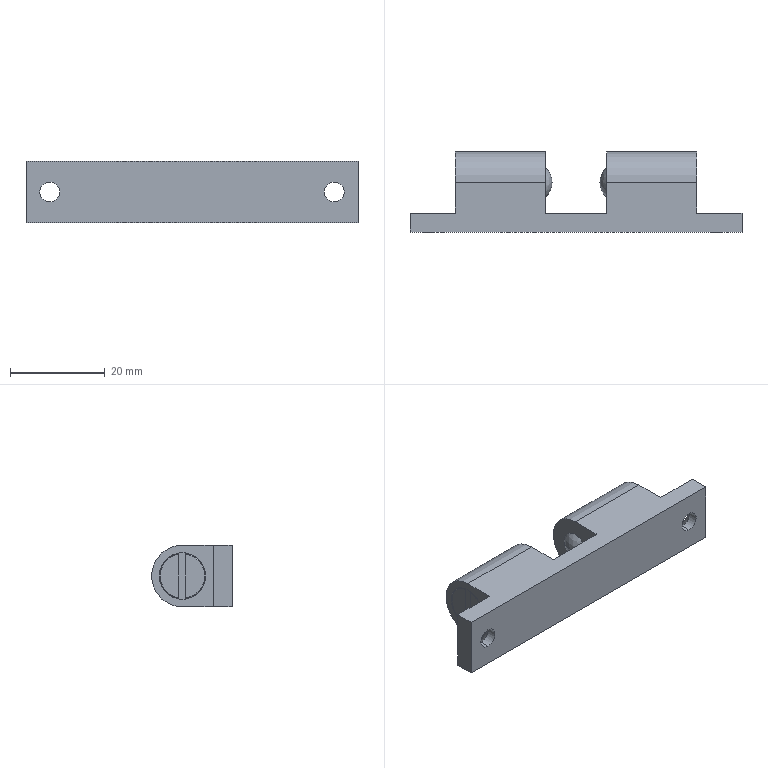Part | STEP file | CATCHE1_MISUMI_BCAS70_Latch | 1 solid | 54 faces | box 70 x 17 x 13 mm | volume 9236 mm3 | plane 22 | cylinder 18 | torus 6 | cone 4 | sphere 4 | commonest cylinder face diameters 9.6 x6 4.2 x4 9.8 x4 0.5 x2 13 x2